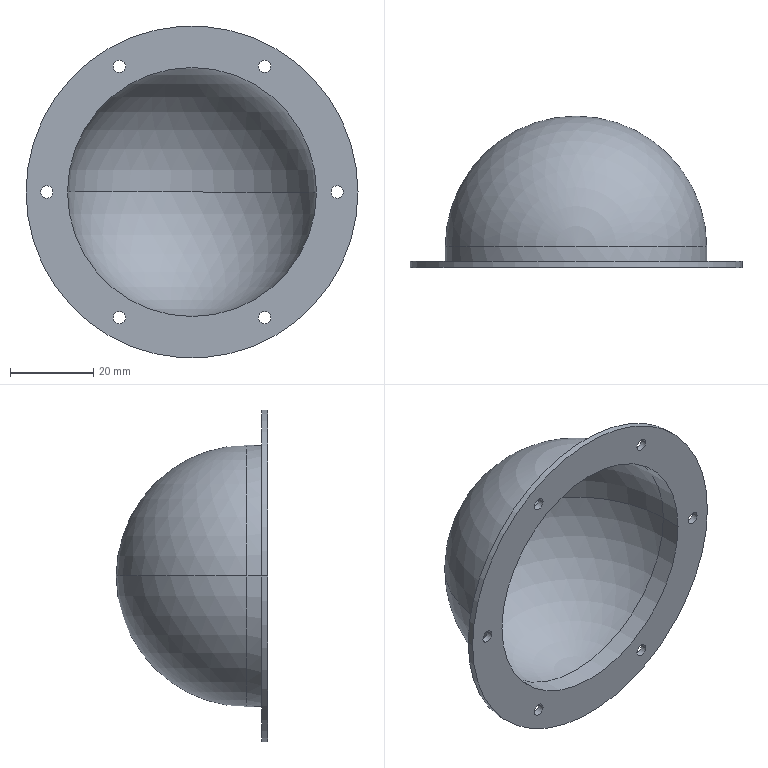Part | SolidWorks | features ICE 1, Revolution 1 | 1 solid | 24 faces | box 80 x 36.5 x 80 mm | volume 13163 mm3 | cylinder 18 | sphere 4 | plane 2 | commonest cylinder face diameters 3 x12 60 x2 63 x2 80 x2
STEP:
#1=CARTESIAN_POINT('',(-16.,0.,-30.311));
#2=VERTEX_POINT('',#1);
#3=CARTESIAN_POINT('',(-19.,0.,-30.311));
#4=VERTEX_POINT('',#3);
#5=CARTESIAN_POINT('',(-17.5,0.,-30.311));
#6=DIRECTION('',(0.,1.,0.));
#7=DIRECTION('',(-1.,0.,0.));
#8=AXIS2_PLACEMENT_3D('',#5,#6,#7);
#9=CIRCLE('',#8,1.5);
#10=EDGE_CURVE('',#2,#4,#9,.T.);
#11=ORIENTED_EDGE('',*,*,#10,.F.);
#12=CARTESIAN_POINT('',(-16.,1.5,-30.311));
#13=VERTEX_POINT('',#12);
#14=CARTESIAN_POINT('',(-16.,0.,-30.311));
#15=DIRECTION('',(0.,1.,0.));
#16=VECTOR('',#15,1000.);
#17=LINE('',#14,#16);
#18=EDGE_CURVE('',#2,#13,#17,.T.);
#19=ORIENTED_EDGE('',*,*,#18,.T.);
#20=CARTESIAN_POINT('',(-19.,1.5,-30.311));
#21=VERTEX_POINT('',#20);
#22=CARTESIAN_POINT('',(-17.5,1.5,-30.311));
#23=DIRECTION('',(0.,1.,0.));
#24=DIRECTION('',(-1.,0.,0.));
#25=AXIS2_PLACEMENT_3D('',#22,#23,#24);
#26=CIRCLE('',#25,1.5);
#27=EDGE_CURVE('',#13,#21,#26,.T.);
#28=ORIENTED_EDGE('',*,*,#27,.T.);
#29=CARTESIAN_POINT('',(-19.,0.,-30.311));
#30=DIRECTION('',(0.,1.,0.));
#31=VECTOR('',#30,1000.);
#32=LINE('',#29,#31);
#33=EDGE_CURVE('',#4,#21,#32,.T.);
#34=ORIENTED_EDGE('',*,*,#33,.F.);
#35=EDGE_LOOP('',(#11,#19,#28,#34));
#36=FACE_OUTER_BOUND('',#35,.T.);
#37=CARTESIAN_POINT('',(-17.5,0.,-30.311));
#38=DIRECTION('',(0.,1.,0.));
#39=DIRECTION('',(-1.,0.,0.));
#40=AXIS2_PLACEMENT_3D('',#37,#38,#39);
#41=CYLINDRICAL_SURFACE('',#40,1.5);
#42=ADVANCED_FACE('',(#36),#41,.F.);
#43=CARTESIAN_POINT('',(19.,0.,-30.311));
#44=VERTEX_POINT('',#43);
#45=CARTESIAN_POINT('',(16.,0.,-30.311));
#46=VERTEX_POINT('',#45);
#47=CARTESIAN_POINT('',(17.5,0.,-30.311));
#48=DIRECTION('',(0.,1.,0.));
#49=DIRECTION('',(-1.,0.,0.));
#50=AXIS2_PLACEMENT_3D('',#47,#48,#49);
#51=CIRCLE('',#50,1.5);
#52=EDGE_CURVE('',#44,#46,#51,.T.);
#53=ORIENTED_EDGE('',*,*,#52,.F.);
#54=CARTESIAN_POINT('',(19.,1.5,-30.311));
#55=VERTEX_POINT('',#54);
#56=CARTESIAN_POINT('',(19.,0.,-30.311));
#57=DIRECTION('',(0.,1.,0.));
#58=VECTOR('',#57,1000.);
#59=LINE('',#56,#58);
#60=EDGE_CURVE('',#44,#55,#59,.T.);
#61=ORIENTED_EDGE('',*,*,#60,.T.);
#62=CARTESIAN_POINT('',(16.,1.5,-30.311));
#63=VERTEX_POINT('',#62);
#64=CARTESIAN_POINT('',(17.5,1.5,-30.311));
#65=DIRECTION('',(0.,1.,0.));
#66=DIRECTION('',(-1.,0.,0.));
#67=AXIS2_PLACEMENT_3D('',#64,#65,#66);
#68=CIRCLE('',#67,1.5);
#69=EDGE_CURVE('',#55,#63,#68,.T.);
#70=ORIENTED_EDGE('',*,*,#69,.T.);
#71=CARTESIAN_POINT('',(16.,0.,-30.311));
#72=DIRECTION('',(0.,1.,0.));
#73=VECTOR('',#72,1000.);
#74=LINE('',#71,#73);
#75=EDGE_CURVE('',#46,#63,#74,.T.);
#76=ORIENTED_EDGE('',*,*,#75,.F.);
#77=EDGE_LOOP('',(#53,#61,#70,#76));
#78=FACE_OUTER_BOUND('',#77,.T.);
#79=CARTESIAN_POINT('',(17.5,0.,-30.311));
#80=DIRECTION('',(0.,1.,0.));
#81=DIRECTION('',(-1.,0.,0.));
#82=AXIS2_PLACEMENT_3D('',#79,#80,#81);
#83=CYLINDRICAL_SURFACE('',#82,1.5);
#84=ADVANCED_FACE('',(#78),#83,.F.);
#85=CARTESIAN_POINT('',(36.5,0.,0.));
#86=VERTEX_POINT('',#85);
#87=CARTESIAN_POINT('',(33.5,0.,0.));
#88=VERTEX_POINT('',#87);
#89=CARTESIAN_POINT('',(35.,0.,0.));
#90=DIRECTION('',(0.,1.,0.));
#91=DIRECTION('',(-1.,0.,0.));
#92=AXIS2_PLACEMENT_3D('',#89,#90,#91);
#93=CIRCLE('',#92,1.5);
#94=EDGE_CURVE('',#86,#88,#93,.T.);
#95=ORIENTED_EDGE('',*,*,#94,.F.);
#96=CARTESIAN_POINT('',(36.5,1.5,0.));
#97=VERTEX_POINT('',#96);
#98=CARTESIAN_POINT('',(36.5,0.,0.));
#99=DIRECTION('',(0.,1.,0.));
#100=VECTOR('',#99,1000.);
#101=LINE('',#98,#100);
#102=EDGE_CURVE('',#86,#97,#101,.T.);
#103=ORIENTED_EDGE('',*,*,#102,.T.);
#104=CARTESIAN_POINT('',(33.5,1.5,0.));
#105=VERTEX_POINT('',#104);
#106=CARTESIAN_POINT('',(35.,1.5,0.));
#107=DIRECTION('',(0.,1.,0.));
#108=DIRECTION('',(-1.,0.,0.));
#109=AXIS2_PLACEMENT_3D('',#106,#107,#108);
#110=CIRCLE('',#109,1.5);
#111=EDGE_CURVE('',#97,#105,#110,.T.);
#112=ORIENTED_EDGE('',*,*,#111,.T.);
#113=CARTESIAN_POINT('',(33.5,0.,0.));
#114=DIRECTION('',(0.,1.,0.));
#115=VECTOR('',#114,1000.);
#116=LINE('',#113,#115);
#117=EDGE_CURVE('',#88,#105,#116,.T.);
#118=ORIENTED_EDGE('',*,*,#117,.F.);
#119=EDGE_LOOP('',(#95,#103,#112,#118));
#120=FACE_OUTER_BOUND('',#119,.T.);
#121=CARTESIAN_POINT('',(35.,0.,0.));
#122=DIRECTION('',(0.,1.,0.));
#123=DIRECTION('',(-1.,0.,0.));
#124=AXIS2_PLACEMENT_3D('',#121,#122,#123);
#125=CYLINDRICAL_SURFACE('',#124,1.5);
#126=ADVANCED_FACE('',(#120),#125,.F.);
#127=CARTESIAN_POINT('',(19.,0.,30.311));
#128=VERTEX_POINT('',#127);
#129=CARTESIAN_POINT('',(16.,0.,30.311));
#130=VERTEX_POINT('',#129);
#131=CARTESIAN_POINT('',(17.5,0.,30.311));
#132=DIRECTION('',(0.,1.,0.));
#133=DIRECTION('',(-1.,0.,0.));
#134=AXIS2_PLACEMENT_3D('',#131,#132,#133);
#135=CIRCLE('',#134,1.5);
#136=EDGE_CURVE('',#128,#130,#135,.T.);
#137=ORIENTED_EDGE('',*,*,#136,.F.);
#138=CARTESIAN_POINT('',(19.,1.5,30.311));
#139=VERTEX_POINT('',#138);
#140=CARTESIAN_POINT('',(19.,0.,30.311));
#141=DIRECTION('',(0.,1.,0.));
#142=VECTOR('',#141,1000.);
#143=LINE('',#140,#142);
#144=EDGE_CURVE('',#128,#139,#143,.T.);
#145=ORIENTED_EDGE('',*,*,#144,.T.);
#146=CARTESIAN_POINT('',(16.,1.5,30.311));
#147=VERTEX_POINT('',#146);
#148=CARTESIAN_POINT('',(17.5,1.5,30.311));
#149=DIRECTION('',(0.,1.,0.));
#150=DIRECTION('',(-1.,0.,0.));
#151=AXIS2_PLACEMENT_3D('',#148,#149,#150);
#152=CIRCLE('',#151,1.5);
#153=EDGE_CURVE('',#139,#147,#152,.T.);
#154=ORIENTED_EDGE('',*,*,#153,.T.);
#155=CARTESIAN_POINT('',(16.,0.,30.311));
#156=DIRECTION('',(0.,1.,0.));
#157=VECTOR('',#156,1000.);
#158=LINE('',#155,#157);
#159=EDGE_CURVE('',#130,#147,#158,.T.);
#160=ORIENTED_EDGE('',*,*,#159,.F.);
#161=EDGE_LOOP('',(#137,#145,#154,#160));
#162=FACE_OUTER_BOUND('',#161,.T.);
#163=CARTESIAN_POINT('',(17.5,0.,30.311));
#164=DIRECTION('',(0.,1.,0.));
#165=DIRECTION('',(-1.,0.,0.));
#166=AXIS2_PLACEMENT_3D('',#163,#164,#165);
#167=CYLINDRICAL_SURFACE('',#166,1.5);
#168=ADVANCED_FACE('',(#162),#167,.F.);
#169=CARTESIAN_POINT('',(-16.,0.,30.311));
#170=VERTEX_POINT('',#169);
#171=CARTESIAN_POINT('',(-19.,0.,30.311));
#172=VERTEX_POINT('',#171);
#173=CARTESIAN_POINT('',(-17.5,0.,30.311));
#174=DIRECTION('',(0.,1.,0.));
#175=DIRECTION('',(-1.,0.,0.));
#176=AXIS2_PLACEMENT_3D('',#173,#174,#175);
#177=CIRCLE('',#176,1.5);
#178=EDGE_CURVE('',#170,#172,#177,.T.);
#179=ORIENTED_EDGE('',*,*,#178,.F.);
#180=CARTESIAN_POINT('',(-16.,1.5,30.311));
#181=VERTEX_POINT('',#180);
#182=CARTESIAN_POINT('',(-16.,0.,30.311));
#183=DIRECTION('',(0.,1.,0.));
#184=VECTOR('',#183,1000.);
#185=LINE('',#182,#184);
#186=EDGE_CURVE('',#170,#181,#185,.T.);
#187=ORIENTED_EDGE('',*,*,#186,.T.);
#188=CARTESIAN_POINT('',(-19.,1.5,30.311));
#189=VERTEX_POINT('',#188);
#190=CARTESIAN_POINT('',(-17.5,1.5,30.311));
#191=DIRECTION('',(0.,1.,0.));
#192=DIRECTION('',(-1.,0.,0.));
#193=AXIS2_PLACEMENT_3D('',#190,#191,#192);
#194=CIRCLE('',#193,1.5);
#195=EDGE_CURVE('',#181,#189,#194,.T.);
#196=ORIENTED_EDGE('',*,*,#195,.T.);
#197=CARTESIAN_POINT('',(-19.,0.,30.311));
#198=DIRECTION('',(0.,1.,0.));
#199=VECTOR('',#198,1000.);
#200=LINE('',#197,#199);
#201=EDGE_CURVE('',#172,#189,#200,.T.);
#202=ORIENTED_EDGE('',*,*,#201,.F.);
#203=EDGE_LOOP('',(#179,#187,#196,#202));
#204=FACE_OUTER_BOUND('',#203,.T.);
#205=CARTESIAN_POINT('',(-17.5,0.,30.311));
#206=DIRECTION('',(0.,1.,0.));
#207=DIRECTION('',(-1.,0.,0.));
#208=AXIS2_PLACEMENT_3D('',#205,#206,#207);
#209=CYLINDRICAL_SURFACE('',#208,1.5);
#210=ADVANCED_FACE('',(#204),#209,.F.);
#211=CARTESIAN_POINT('',(-33.5,0.,0.));
#212=VERTEX_POINT('',#211);
#213=CARTESIAN_POINT('',(-36.5,0.,0.));
#214=VERTEX_POINT('',#213);
#215=CARTESIAN_POINT('',(-35.,0.,0.));
#216=DIRECTION('',(0.,1.,0.));
#217=DIRECTION('',(-1.,0.,0.));
#218=AXIS2_PLACEMENT_3D('',#215,#216,#217);
#219=CIRCLE('',#218,1.5);
#220=EDGE_CURVE('',#212,#214,#219,.T.);
#221=ORIENTED_EDGE('',*,*,#220,.F.);
#222=CARTESIAN_POINT('',(-33.5,1.5,0.));
#223=VERTEX_POINT('',#222);
#224=CARTESIAN_POINT('',(-33.5,0.,0.));
#225=DIRECTION('',(0.,1.,0.));
#226=VECTOR('',#225,1000.);
#227=LINE('',#224,#226);
#228=EDGE_CURVE('',#212,#223,#227,.T.);
#229=ORIENTED_EDGE('',*,*,#228,.T.);
#230=CARTESIAN_POINT('',(-36.5,1.5,0.));
#231=VERTEX_POINT('',#230);
#232=CARTESIAN_POINT('',(-35.,1.5,0.));
#233=DIRECTION('',(0.,1.,0.));
#234=DIRECTION('',(-1.,0.,0.));
#235=AXIS2_PLACEMENT_3D('',#232,#233,#234);
#236=CIRCLE('',#235,1.5);
#237=EDGE_CURVE('',#223,#231,#236,.T.);
#238=ORIENTED_EDGE('',*,*,#237,.T.);
#239=CARTESIAN_POINT('',(-36.5,0.,0.));
#240=DIRECTION('',(0.,1.,0.));
#241=VECTOR('',#240,1000.);
#242=LINE('',#239,#241);
#243=EDGE_CURVE('',#214,#231,#242,.T.);
#244=ORIENTED_EDGE('',*,*,#243,.F.);
#245=EDGE_LOOP('',(#221,#229,#238,#244));
#246=FACE_OUTER_BOUND('',#245,.T.);
#247=CARTESIAN_POINT('',(-35.,0.,0.));
#248=DIRECTION('',(0.,1.,0.));
#249=DIRECTION('',(-1.,0.,0.));
#250=AXIS2_PLACEMENT_3D('',#247,#248,#249);
#251=CYLINDRICAL_SURFACE('',#250,1.5);
#252=ADVANCED_FACE('',(#246),#251,.F.);
#253=CARTESIAN_POINT('',(-30.,5.,0.));
#254=VERTEX_POINT('',#253);
#255=CARTESIAN_POINT('',(30.,5.,0.));
#256=VERTEX_POINT('',#255);
#257=CARTESIAN_POINT('',(0.,5.,0.));
#258=DIRECTION('',(0.,-1.,0.));
#259=DIRECTION('',(1.,0.,0.));
#260=AXIS2_PLACEMENT_3D('',#257,#258,#259);
#261=CIRCLE('',#260,30.);
#262=EDGE_CURVE('',#254,#256,#261,.T.);
#263=ORIENTED_EDGE('',*,*,#262,.F.);
#264=CARTESIAN_POINT('',(-30.,0.,0.));
#265=VERTEX_POINT('',#264);
#266=CARTESIAN_POINT('',(-30.,35.,0.));
#267=DIRECTION('',(0.,-1.,0.));
#268=VECTOR('',#267,1000.);
#269=LINE('',#266,#268);
#270=EDGE_CURVE('',#254,#265,#269,.T.);
#271=ORIENTED_EDGE('',*,*,#270,.T.);
#272=CARTESIAN_POINT('',(30.,0.,0.));
#273=VERTEX_POINT('',#272);
#274=CARTESIAN_POINT('',(0.,0.,0.));
#275=DIRECTION('',(0.,-1.,0.));
#276=DIRECTION('',(1.,0.,0.));
#277=AXIS2_PLACEMENT_3D('',#274,#275,#276);
#278=CIRCLE('',#277,30.);
#279=EDGE_CURVE('',#265,#273,#278,.T.);
#280=ORIENTED_EDGE('',*,*,#279,.T.);
#281=CARTESIAN_POINT('',(30.,35.,0.));
#282=DIRECTION('',(0.,-1.,0.));
#283=VECTOR('',#282,1000.);
#284=LINE('',#281,#283);
#285=EDGE_CURVE('',#256,#273,#284,.T.);
#286=ORIENTED_EDGE('',*,*,#285,.F.);
#287=EDGE_LOOP('',(#263,#271,#280,#286));
#288=FACE_OUTER_BOUND('',#287,.T.);
#289=CARTESIAN_POINT('',(0.,35.,0.));
#290=DIRECTION('',(0.,-1.,0.));
#291=DIRECTION('',(1.,0.,0.));
#292=AXIS2_PLACEMENT_3D('',#289,#290,#291);
#293=CYLINDRICAL_SURFACE('',#292,30.);
#294=ADVANCED_FACE('',(#288),#293,.F.);
#295=CARTESIAN_POINT('',(40.,1.5,0.));
#296=VERTEX_POINT('',#295);
#297=CARTESIAN_POINT('',(-40.,1.5,0.));
#298=VERTEX_POINT('',#297);
#299=CARTESIAN_POINT('',(0.,1.5,0.));
#300=DIRECTION('',(0.,-1.,0.));
#301=DIRECTION('',(1.,0.,0.));
#302=AXIS2_PLACEMENT_3D('',#299,#300,#301);
#303=CIRCLE('',#302,40.);
#304=EDGE_CURVE('',#296,#298,#303,.T.);
#305=ORIENTED_EDGE('',*,*,#304,.T.);
#306=CARTESIAN_POINT('',(-40.,0.,0.));
#307=VERTEX_POINT('',#306);
#308=CARTESIAN_POINT('',(-40.,35.,0.));
#309=DIRECTION('',(0.,-1.,0.));
#310=VECTOR('',#309,1000.);
#311=LINE('',#308,#310);
#312=EDGE_CURVE('',#298,#307,#311,.T.);
#313=ORIENTED_EDGE('',*,*,#312,.T.);
#314=CARTESIAN_POINT('',(40.,0.,0.));
#315=VERTEX_POINT('',#314);
#316=CARTESIAN_POINT('',(0.,0.,0.));
#317=DIRECTION('',(0.,-1.,0.));
#318=DIRECTION('',(1.,0.,0.));
#319=AXIS2_PLACEMENT_3D('',#316,#317,#318);
#320=CIRCLE('',#319,40.);
#321=EDGE_CURVE('',#315,#307,#320,.T.);
#322=ORIENTED_EDGE('',*,*,#321,.F.);
#323=CARTESIAN_POINT('',(40.,35.,0.));
#324=DIRECTION('',(0.,-1.,0.));
#325=VECTOR('',#324,1000.);
#326=LINE('',#323,#325);
#327=EDGE_CURVE('',#296,#315,#326,.T.);
#328=ORIENTED_EDGE('',*,*,#327,.F.);
#329=EDGE_LOOP('',(#305,#313,#322,#328));
#330=FACE_OUTER_BOUND('',#329,.T.);
#331=CARTESIAN_POINT('',(0.,35.,0.));
#332=DIRECTION('',(0.,-1.,0.));
#333=DIRECTION('',(1.,0.,0.));
#334=AXIS2_PLACEMENT_3D('',#331,#332,#333);
#335=CYLINDRICAL_SURFACE('',#334,40.);
#336=ADVANCED_FACE('',(#330),#335,.T.);
#337=CARTESIAN_POINT('',(31.5,5.,0.));
#338=VERTEX_POINT('',#337);
#339=CARTESIAN_POINT('',(-31.5,5.,0.));
#340=VERTEX_POINT('',#339);
#341=CARTESIAN_POINT('',(0.,5.,0.));
#342=DIRECTION('',(0.,-1.,0.));
#343=DIRECTION('',(1.,0.,0.));
#344=AXIS2_PLACEMENT_3D('',#341,#342,#343);
#345=CIRCLE('',#344,31.5);
#346=EDGE_CURVE('',#338,#340,#345,.T.);
#347=ORIENTED_EDGE('',*,*,#346,.T.);
#348=CARTESIAN_POINT('',(-31.5,1.5,0.));
#349=VERTEX_POINT('',#348);
#350=CARTESIAN_POINT('',(-31.5,35.,0.));
#351=DIRECTION('',(0.,-1.,0.));
#352=VECTOR('',#351,1000.);
#353=LINE('',#350,#352);
#354=EDGE_CURVE('',#340,#349,#353,.T.);
#355=ORIENTED_EDGE('',*,*,#354,.T.);
#356=CARTESIAN_POINT('',(31.5,1.5,0.));
#357=VERTEX_POINT('',#356);
#358=CARTESIAN_POINT('',(0.,1.5,0.));
#359=DIRECTION('',(0.,-1.,0.));
#360=DIRECTION('',(1.,0.,0.));
#361=AXIS2_PLACEMENT_3D('',#358,#359,#360);
#362=CIRCLE('',#361,31.5);
#363=EDGE_CURVE('',#357,#349,#362,.T.);
#364=ORIENTED_EDGE('',*,*,#363,.F.);
#365=CARTESIAN_POINT('',(31.5,35.,0.));
#366=DIRECTION('',(0.,-1.,0.));
#367=VECTOR('',#366,1000.);
#368=LINE('',#365,#367);
#369=EDGE_CURVE('',#338,#357,#368,.T.);
#370=ORIENTED_EDGE('',*,*,#369,.F.);
#371=EDGE_LOOP('',(#347,#355,#364,#370));
#372=FACE_OUTER_BOUND('',#371,.T.);
#373=CARTESIAN_POINT('',(0.,35.,0.));
#374=DIRECTION('',(0.,-1.,0.));
#375=DIRECTION('',(1.,0.,0.));
#376=AXIS2_PLACEMENT_3D('',#373,#374,#375);
#377=CYLINDRICAL_SURFACE('',#376,31.5);
#378=ADVANCED_FACE('',(#372),#377,.T.);
#379=CARTESIAN_POINT('',(0.,36.5,0.));
#380=VERTEX_POINT('',#379);
#381=CARTESIAN_POINT('',(0.,5.,0.));
#382=DIRECTION('',(0.,0.,1.));
#383=DIRECTION('',(1.,0.,0.));
#384=AXIS2_PLACEMENT_3D('',#381,#382,#383);
#385=CIRCLE('',#384,31.5);
#386=EDGE_CURVE('',#380,#340,#385,.T.);
#387=ORIENTED_EDGE('',*,*,#386,.F.);
#388=CARTESIAN_POINT('',(0.,5.,0.));
#389=DIRECTION('',(0.,0.,-1.));
#390=DIRECTION('',(-1.,0.,0.));
#391=AXIS2_PLACEMENT_3D('',#388,#389,#390);
#392=CIRCLE('',#391,31.5);
#393=EDGE_CURVE('',#380,#338,#392,.T.);
#394=ORIENTED_EDGE('',*,*,#393,.T.);
#395=CARTESIAN_POINT('',(0.,5.,0.));
#396=DIRECTION('',(0.,-1.,0.));
#397=DIRECTION('',(1.,0.,0.));
#398=AXIS2_PLACEMENT_3D('',#395,#396,#397);
#399=CIRCLE('',#398,31.5);
#400=EDGE_CURVE('',#340,#338,#399,.T.);
#401=ORIENTED_EDGE('',*,*,#400,.F.);
#402=EDGE_LOOP('',(#387,#394,#401));
#403=FACE_OUTER_BOUND('',#402,.T.);
#404=CARTESIAN_POINT('',(0.,5.,0.));
#405=DIRECTION('',(0.,0.,-1.));
#406=DIRECTION('',(-1.,0.,0.));
#407=AXIS2_PLACEMENT_3D('',#404,#405,#406);
#408=SPHERICAL_SURFACE('',#407,31.5);
#409=ADVANCED_FACE('',(#403),#408,.T.);
#410=CARTESIAN_POINT('',(0.,35.,0.));
#411=VERTEX_POINT('',#410);
#412=CARTESIAN_POINT('',(0.,5.,0.));
#413=DIRECTION('',(0.,0.,1.));
#414=DIRECTION('',(1.,0.,0.));
#415=AXIS2_PLACEMENT_3D('',#412,#413,#414);
#416=CIRCLE('',#415,30.);
#417=EDGE_CURVE('',#411,#254,#416,.T.);
#418=ORIENTED_EDGE('',*,*,#417,.F.);
#419=CARTESIAN_POINT('',(0.,5.,0.));
#420=DIRECTION('',(0.,0.,-1.));
#421=DIRECTION('',(-1.,0.,0.));
#422=AXIS2_PLACEMENT_3D('',#419,#420,#421);
#423=CIRCLE('',#422,30.);
#424=EDGE_CURVE('',#411,#256,#423,.T.);
#425=ORIENTED_EDGE('',*,*,#424,.T.);
#426=CARTESIAN_POINT('',(0.,5.,0.));
#427=DIRECTION('',(0.,-1.,0.));
#428=DIRECTION('',(1.,0.,0.));
#429=AXIS2_PLACEMENT_3D('',#426,#427,#428);
#430=CIRCLE('',#429,30.);
#431=EDGE_CURVE('',#256,#254,#430,.T.);
#432=ORIENTED_EDGE('',*,*,#431,.T.);
#433=EDGE_LOOP('',(#418,#425,#432));
#434=FACE_OUTER_BOUND('',#433,.T.);
#435=CARTESIAN_POINT('',(0.,5.,0.));
#436=DIRECTION('',(0.,0.,-1.));
#437=DIRECTION('',(-1.,0.,0.));
#438=AXIS2_PLACEMENT_3D('',#435,#436,#437);
#439=SPHERICAL_SURFACE('',#438,30.);
#440=ADVANCED_FACE('',(#434),#439,.F.);
#441=ORIENTED_EDGE('',*,*,#424,.F.);
#442=ORIENTED_EDGE('',*,*,#417,.T.);
#443=ORIENTED_EDGE('',*,*,#262,.T.);
#444=EDGE_LOOP('',(#441,#442,#443));
#445=FACE_OUTER_BOUND('',#444,.T.);
#446=CARTESIAN_POINT('',(0.,5.,0.));
#447=DIRECTION('',(0.,0.,-1.));
#448=DIRECTION('',(-1.,0.,0.));
#449=AXIS2_PLACEMENT_3D('',#446,#447,#448);
#450=SPHERICAL_SURFACE('',#449,30.);
#451=ADVANCED_FACE('',(#445),#450,.F.);
#452=ORIENTED_EDGE('',*,*,#393,.F.);
#453=ORIENTED_EDGE('',*,*,#386,.T.);
#454=ORIENTED_EDGE('',*,*,#346,.F.);
#455=EDGE_LOOP('',(#452,#453,#454));
#456=FACE_OUTER_BOUND('',#455,.T.);
#457=CARTESIAN_POINT('',(0.,5.,0.));
#458=DIRECTION('',(0.,0.,-1.));
#459=DIRECTION('',(-1.,0.,0.));
#460=AXIS2_PLACEMENT_3D('',#457,#458,#459);
#461=SPHERICAL_SURFACE('',#460,31.5);
#462=ADVANCED_FACE('',(#456),#461,.T.);
#463=ORIENTED_EDGE('',*,*,#354,.F.);
#464=ORIENTED_EDGE('',*,*,#400,.T.);
#465=ORIENTED_EDGE('',*,*,#369,.T.);
#466=CARTESIAN_POINT('',(0.,1.5,0.));
#467=DIRECTION('',(0.,-1.,0.));
#468=DIRECTION('',(1.,0.,0.));
#469=AXIS2_PLACEMENT_3D('',#466,#467,#468);
#470=CIRCLE('',#469,31.5);
#471=EDGE_CURVE('',#349,#357,#470,.T.);
#472=ORIENTED_EDGE('',*,*,#471,.F.);
#473=EDGE_LOOP('',(#463,#464,#465,#472));
#474=FACE_OUTER_BOUND('',#473,.T.);
#475=CARTESIAN_POINT('',(0.,35.,0.));
#476=DIRECTION('',(0.,-1.,0.));
#477=DIRECTION('',(1.,0.,0.));
#478=AXIS2_PLACEMENT_3D('',#475,#476,#477);
#479=CYLINDRICAL_SURFACE('',#478,31.5);
#480=ADVANCED_FACE('',(#474),#479,.T.);
#481=CARTESIAN_POINT('',(-17.5,1.5,-30.311));
#482=DIRECTION('',(0.,1.,0.));
#483=DIRECTION('',(-1.,0.,0.));
#484=AXIS2_PLACEMENT_3D('',#481,#482,#483);
#485=CIRCLE('',#484,1.5);
#486=EDGE_CURVE('',#21,#13,#485,.T.);
#487=ORIENTED_EDGE('',*,*,#486,.F.);
#488=ORIENTED_EDGE('',*,*,#27,.F.);
#489=EDGE_LOOP('',(#487,#488));
#490=FACE_BOUND('',#489,.T.);
#491=CARTESIAN_POINT('',(17.5,1.5,-30.311));
#492=DIRECTION('',(0.,1.,0.));
#493=DIRECTION('',(-1.,0.,0.));
#494=AXIS2_PLACEMENT_3D('',#491,#492,#493);
#495=CIRCLE('',#494,1.5);
#496=EDGE_CURVE('',#63,#55,#495,.T.);
#497=ORIENTED_EDGE('',*,*,#496,.F.);
#498=ORIENTED_EDGE('',*,*,#69,.F.);
#499=EDGE_LOOP('',(#497,#498));
#500=FACE_BOUND('',#499,.T.);
#501=CARTESIAN_POINT('',(35.,1.5,0.));
#502=DIRECTION('',(0.,1.,0.));
#503=DIRECTION('',(-1.,0.,0.));
#504=AXIS2_PLACEMENT_3D('',#501,#502,#503);
#505=CIRCLE('',#504,1.5);
#506=EDGE_CURVE('',#105,#97,#505,.T.);
#507=ORIENTED_EDGE('',*,*,#506,.F.);
#508=ORIENTED_EDGE('',*,*,#111,.F.);
#509=EDGE_LOOP('',(#507,#508));
#510=FACE_BOUND('',#509,.T.);
#511=CARTESIAN_POINT('',(17.5,1.5,30.311));
#512=DIRECTION('',(0.,1.,0.));
#513=DIRECTION('',(-1.,0.,0.));
#514=AXIS2_PLACEMENT_3D('',#511,#512,#513);
#515=CIRCLE('',#514,1.5);
#516=EDGE_CURVE('',#147,#139,#515,.T.);
#517=ORIENTED_EDGE('',*,*,#516,.F.);
#518=ORIENTED_EDGE('',*,*,#153,.F.);
#519=EDGE_LOOP('',(#517,#518));
#520=FACE_BOUND('',#519,.T.);
#521=CARTESIAN_POINT('',(-17.5,1.5,30.311));
#522=DIRECTION('',(0.,1.,0.));
#523=DIRECTION('',(-1.,0.,0.));
#524=AXIS2_PLACEMENT_3D('',#521,#522,#523);
#525=CIRCLE('',#524,1.5);
#526=EDGE_CURVE('',#189,#181,#525,.T.);
#527=ORIENTED_EDGE('',*,*,#526,.F.);
#528=ORIENTED_EDGE('',*,*,#195,.F.);
#529=EDGE_LOOP('',(#527,#528));
#530=FACE_BOUND('',#529,.T.);
#531=CARTESIAN_POINT('',(-35.,1.5,0.));
#532=DIRECTION('',(0.,1.,0.));
#533=DIRECTION('',(-1.,0.,0.));
#534=AXIS2_PLACEMENT_3D('',#531,#532,#533);
#535=CIRCLE('',#534,1.5);
#536=EDGE_CURVE('',#231,#223,#535,.T.);
#537=ORIENTED_EDGE('',*,*,#536,.F.);
#538=ORIENTED_EDGE('',*,*,#237,.F.);
#539=EDGE_LOOP('',(#537,#538));
#540=FACE_BOUND('',#539,.T.);
#541=ORIENTED_EDGE('',*,*,#304,.F.);
#542=CARTESIAN_POINT('',(0.,1.5,0.));
#543=DIRECTION('',(0.,-1.,0.));
#544=DIRECTION('',(1.,0.,0.));
#545=AXIS2_PLACEMENT_3D('',#542,#543,#544);
#546=CIRCLE('',#545,40.);
#547=EDGE_CURVE('',#298,#296,#546,.T.);
#548=ORIENTED_EDGE('',*,*,#547,.F.);
#549=EDGE_LOOP('',(#541,#548));
#550=FACE_OUTER_BOUND('',#549,.T.);
#551=ORIENTED_EDGE('',*,*,#363,.T.);
#552=ORIENTED_EDGE('',*,*,#471,.T.);
#553=EDGE_LOOP('',(#551,#552));
#554=FACE_BOUND('',#553,.T.);
#555=CARTESIAN_POINT('',(-40.,1.5,0.));
#556=DIRECTION('',(0.,-1.,0.));
#557=DIRECTION('',(1.,0.,0.));
#558=AXIS2_PLACEMENT_3D('',#555,#556,#557);
#559=PLANE('',#558);
#560=ADVANCED_FACE('',(#490,#500,#510,#520,#530,#540,#550,#554),#559,.F.);
#561=ORIENTED_EDGE('',*,*,#312,.F.);
#562=ORIENTED_EDGE('',*,*,#547,.T.);
#563=ORIENTED_EDGE('',*,*,#327,.T.);
#564=CARTESIAN_POINT('',(0.,0.,0.));
#565=DIRECTION('',(0.,-1.,0.));
#566=DIRECTION('',(1.,0.,0.));
#567=AXIS2_PLACEMENT_3D('',#564,#565,#566);
#568=CIRCLE('',#567,40.);
#569=EDGE_CURVE('',#307,#315,#568,.T.);
#570=ORIENTED_EDGE('',*,*,#569,.F.);
#571=EDGE_LOOP('',(#561,#562,#563,#570));
#572=FACE_OUTER_BOUND('',#571,.T.);
#573=CARTESIAN_POINT('',(0.,35.,0.));
#574=DIRECTION('',(0.,-1.,0.));
#575=DIRECTION('',(1.,0.,0.));
#576=AXIS2_PLACEMENT_3D('',#573,#574,#575);
#577=CYLINDRICAL_SURFACE('',#576,40.);
#578=ADVANCED_FACE('',(#572),#577,.T.);
#579=CARTESIAN_POINT('',(-17.5,0.,-30.311));
#580=DIRECTION('',(0.,1.,0.));
#581=DIRECTION('',(-1.,0.,0.));
#582=AXIS2_PLACEMENT_3D('',#579,#580,#581);
#583=CIRCLE('',#582,1.5);
#584=EDGE_CURVE('',#4,#2,#583,.T.);
#585=ORIENTED_EDGE('',*,*,#584,.T.);
#586=ORIENTED_EDGE('',*,*,#10,.T.);
#587=EDGE_LOOP('',(#585,#586));
#588=FACE_BOUND('',#587,.T.);
#589=CARTESIAN_POINT('',(17.5,0.,-30.311));
#590=DIRECTION('',(0.,1.,0.));
#591=DIRECTION('',(-1.,0.,0.));
#592=AXIS2_PLACEMENT_3D('',#589,#590,#591);
#593=CIRCLE('',#592,1.5);
#594=EDGE_CURVE('',#46,#44,#593,.T.);
#595=ORIENTED_EDGE('',*,*,#594,.T.);
#596=ORIENTED_EDGE('',*,*,#52,.T.);
#597=EDGE_LOOP('',(#595,#596));
#598=FACE_BOUND('',#597,.T.);
#599=CARTESIAN_POINT('',(35.,0.,0.));
#600=DIRECTION('',(0.,1.,0.));
#601=DIRECTION('',(-1.,0.,0.));
#602=AXIS2_PLACEMENT_3D('',#599,#600,#601);
#603=CIRCLE('',#602,1.5);
#604=EDGE_CURVE('',#88,#86,#603,.T.);
#605=ORIENTED_EDGE('',*,*,#604,.T.);
#606=ORIENTED_EDGE('',*,*,#94,.T.);
#607=EDGE_LOOP('',(#605,#606));
#608=FACE_BOUND('',#607,.T.);
#609=CARTESIAN_POINT('',(17.5,0.,30.311));
#610=DIRECTION('',(0.,1.,0.));
#611=DIRECTION('',(-1.,0.,0.));
#612=AXIS2_PLACEMENT_3D('',#609,#610,#611);
#613=CIRCLE('',#612,1.5);
#614=EDGE_CURVE('',#130,#128,#613,.T.);
#615=ORIENTED_EDGE('',*,*,#614,.T.);
#616=ORIENTED_EDGE('',*,*,#136,.T.);
#617=EDGE_LOOP('',(#615,#616));
#618=FACE_BOUND('',#617,.T.);
#619=CARTESIAN_POINT('',(-17.5,0.,30.311));
#620=DIRECTION('',(0.,1.,0.));
#621=DIRECTION('',(-1.,0.,0.));
#622=AXIS2_PLACEMENT_3D('',#619,#620,#621);
#623=CIRCLE('',#622,1.5);
#624=EDGE_CURVE('',#172,#170,#623,.T.);
#625=ORIENTED_EDGE('',*,*,#624,.T.);
#626=ORIENTED_EDGE('',*,*,#178,.T.);
#627=EDGE_LOOP('',(#625,#626));
#628=FACE_BOUND('',#627,.T.);
#629=CARTESIAN_POINT('',(-35.,0.,0.));
#630=DIRECTION('',(0.,1.,0.));
#631=DIRECTION('',(-1.,0.,0.));
#632=AXIS2_PLACEMENT_3D('',#629,#630,#631);
#633=CIRCLE('',#632,1.5);
#634=EDGE_CURVE('',#214,#212,#633,.T.);
#635=ORIENTED_EDGE('',*,*,#634,.T.);
#636=ORIENTED_EDGE('',*,*,#220,.T.);
#637=EDGE_LOOP('',(#635,#636));
#638=FACE_BOUND('',#637,.T.);
#639=CARTESIAN_POINT('',(0.,0.,0.));
#640=DIRECTION('',(0.,-1.,0.));
#641=DIRECTION('',(1.,0.,0.));
#642=AXIS2_PLACEMENT_3D('',#639,#640,#641);
#643=CIRCLE('',#642,30.);
#644=EDGE_CURVE('',#273,#265,#643,.T.);
#645=ORIENTED_EDGE('',*,*,#644,.F.);
#646=ORIENTED_EDGE('',*,*,#279,.F.);
#647=EDGE_LOOP('',(#645,#646));
#648=FACE_BOUND('',#647,.T.);
#649=ORIENTED_EDGE('',*,*,#321,.T.);
#650=ORIENTED_EDGE('',*,*,#569,.T.);
#651=EDGE_LOOP('',(#649,#650));
#652=FACE_OUTER_BOUND('',#651,.T.);
#653=CARTESIAN_POINT('',(-40.,0.,0.));
#654=DIRECTION('',(0.,1.,0.));
#655=DIRECTION('',(-1.,0.,0.));
#656=AXIS2_PLACEMENT_3D('',#653,#654,#655);
#657=PLANE('',#656);
#658=ADVANCED_FACE('',(#588,#598,#608,#618,#628,#638,#648,#652),#657,.F.);
#659=ORIENTED_EDGE('',*,*,#270,.F.);
#660=ORIENTED_EDGE('',*,*,#431,.F.);
#661=ORIENTED_EDGE('',*,*,#285,.T.);
#662=ORIENTED_EDGE('',*,*,#644,.T.);
#663=EDGE_LOOP('',(#659,#660,#661,#662));
#664=FACE_OUTER_BOUND('',#663,.T.);
#665=CARTESIAN_POINT('',(0.,35.,0.));
#666=DIRECTION('',(0.,-1.,0.));
#667=DIRECTION('',(1.,0.,0.));
#668=AXIS2_PLACEMENT_3D('',#665,#666,#667);
#669=CYLINDRICAL_SURFACE('',#668,30.);
#670=ADVANCED_FACE('',(#664),#669,.F.);
#671=ORIENTED_EDGE('',*,*,#228,.F.);
#672=ORIENTED_EDGE('',*,*,#634,.F.);
#673=ORIENTED_EDGE('',*,*,#243,.T.);
#674=ORIENTED_EDGE('',*,*,#536,.T.);
#675=EDGE_LOOP('',(#671,#672,#673,#674));
#676=FACE_OUTER_BOUND('',#675,.T.);
#677=CARTESIAN_POINT('',(-35.,0.,0.));
#678=DIRECTION('',(0.,1.,0.));
#679=DIRECTION('',(-1.,0.,0.));
#680=AXIS2_PLACEMENT_3D('',#677,#678,#679);
#681=CYLINDRICAL_SURFACE('',#680,1.5);
#682=ADVANCED_FACE('',(#676),#681,.F.);
#683=ORIENTED_EDGE('',*,*,#186,.F.);
#684=ORIENTED_EDGE('',*,*,#624,.F.);
#685=ORIENTED_EDGE('',*,*,#201,.T.);
#686=ORIENTED_EDGE('',*,*,#526,.T.);
#687=EDGE_LOOP('',(#683,#684,#685,#686));
#688=FACE_OUTER_BOUND('',#687,.T.);
#689=CARTESIAN_POINT('',(-17.5,0.,30.311));
#690=DIRECTION('',(0.,1.,0.));
#691=DIRECTION('',(-1.,0.,0.));
#692=AXIS2_PLACEMENT_3D('',#689,#690,#691);
#693=CYLINDRICAL_SURFACE('',#692,1.5);
#694=ADVANCED_FACE('',(#688),#693,.F.);
#695=ORIENTED_EDGE('',*,*,#144,.F.);
#696=ORIENTED_EDGE('',*,*,#614,.F.);
#697=ORIENTED_EDGE('',*,*,#159,.T.);
#698=ORIENTED_EDGE('',*,*,#516,.T.);
#699=EDGE_LOOP('',(#695,#696,#697,#698));
#700=FACE_OUTER_BOUND('',#699,.T.);
#701=CARTESIAN_POINT('',(17.5,0.,30.311));
#702=DIRECTION('',(0.,1.,0.));
#703=DIRECTION('',(-1.,0.,0.));
#704=AXIS2_PLACEMENT_3D('',#701,#702,#703);
#705=CYLINDRICAL_SURFACE('',#704,1.5);
#706=ADVANCED_FACE('',(#700),#705,.F.);
#707=ORIENTED_EDGE('',*,*,#102,.F.);
#708=ORIENTED_EDGE('',*,*,#604,.F.);
#709=ORIENTED_EDGE('',*,*,#117,.T.);
#710=ORIENTED_EDGE('',*,*,#506,.T.);
#711=EDGE_LOOP('',(#707,#708,#709,#710));
#712=FACE_OUTER_BOUND('',#711,.T.);
#713=CARTESIAN_POINT('',(35.,0.,0.));
#714=DIRECTION('',(0.,1.,0.));
#715=DIRECTION('',(-1.,0.,0.));
#716=AXIS2_PLACEMENT_3D('',#713,#714,#715);
#717=CYLINDRICAL_SURFACE('',#716,1.5);
#718=ADVANCED_FACE('',(#712),#717,.F.);
#719=ORIENTED_EDGE('',*,*,#60,.F.);
#720=ORIENTED_EDGE('',*,*,#594,.F.);
#721=ORIENTED_EDGE('',*,*,#75,.T.);
#722=ORIENTED_EDGE('',*,*,#496,.T.);
#723=EDGE_LOOP('',(#719,#720,#721,#722));
#724=FACE_OUTER_BOUND('',#723,.T.);
#725=CARTESIAN_POINT('',(17.5,0.,-30.311));
#726=DIRECTION('',(0.,1.,0.));
#727=DIRECTION('',(-1.,0.,0.));
#728=AXIS2_PLACEMENT_3D('',#725,#726,#727);
#729=CYLINDRICAL_SURFACE('',#728,1.5);
#730=ADVANCED_FACE('',(#724),#729,.F.);
#731=ORIENTED_EDGE('',*,*,#18,.F.);
#732=ORIENTED_EDGE('',*,*,#584,.F.);
#733=ORIENTED_EDGE('',*,*,#33,.T.);
#734=ORIENTED_EDGE('',*,*,#486,.T.);
#735=EDGE_LOOP('',(#731,#732,#733,#734));
#736=FACE_OUTER_BOUND('',#735,.T.);
#737=CARTESIAN_POINT('',(-17.5,0.,-30.311));
#738=DIRECTION('',(0.,1.,0.));
#739=DIRECTION('',(-1.,0.,0.));
#740=AXIS2_PLACEMENT_3D('',#737,#738,#739);
#741=CYLINDRICAL_SURFACE('',#740,1.5);
#742=ADVANCED_FACE('',(#736),#741,.F.);
#743=CLOSED_SHELL('',(#42,#84,#126,#168,#210,#252,#294,#336,#378,#409,#440,#451,#462,#480,#560,#578,#658,#670,#682,#694,#706,#718,#730,#742));
#744=MANIFOLD_SOLID_BREP('',#743);
#745=CARTESIAN_POINT('',(0.,0.,0.));
#746=DIRECTION('',(0.,0.,1.));
#747=DIRECTION('',(1.,0.,0.));
#748=AXIS2_PLACEMENT_3D('',#745,#746,#747);
#749=(LENGTH_UNIT()NAMED_UNIT(*)SI_UNIT(.MILLI.,.METRE.));
#750=UNCERTAINTY_MEASURE_WITH_UNIT(LENGTH_MEASURE(0.00001),#749,'','');
#751=(NAMED_UNIT(*)PLANE_ANGLE_UNIT()SI_UNIT($,.RADIAN.));
#752=(NAMED_UNIT(*)SI_UNIT($,.STERADIAN.)SOLID_ANGLE_UNIT());
#753=(GEOMETRIC_REPRESENTATION_CONTEXT(3)GLOBAL_UNCERTAINTY_ASSIGNED_CONTEXT((#750))GLOBAL_UNIT_ASSIGNED_CONTEXT((#749,#751,#752))REPRESENTATION_CONTEXT('',''));
#754=ADVANCED_BREP_SHAPE_REPRESENTATION('',(#744,#748),#753);